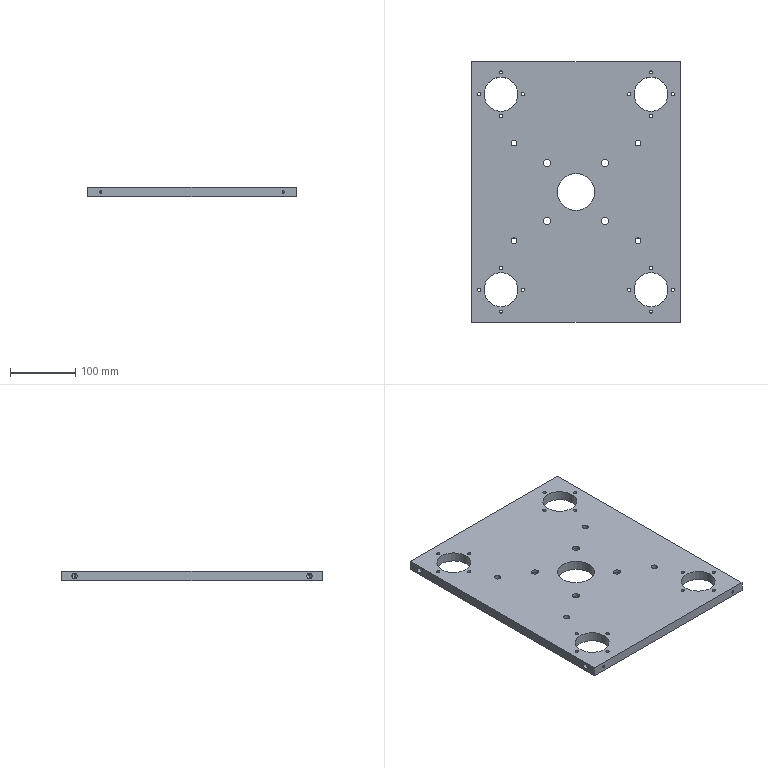Part | STEP file | 44-02-19 Press-fit Push Plate | 1 solid | 108 faces | box 320 x 400 x 15 mm | volume 1729546 mm3 | cylinder 82 | cone 16 | plane 10 | commonest cylinder face diameters 5 x32 3.5 x12 9 x8 11 x8 18 x8 52 x8